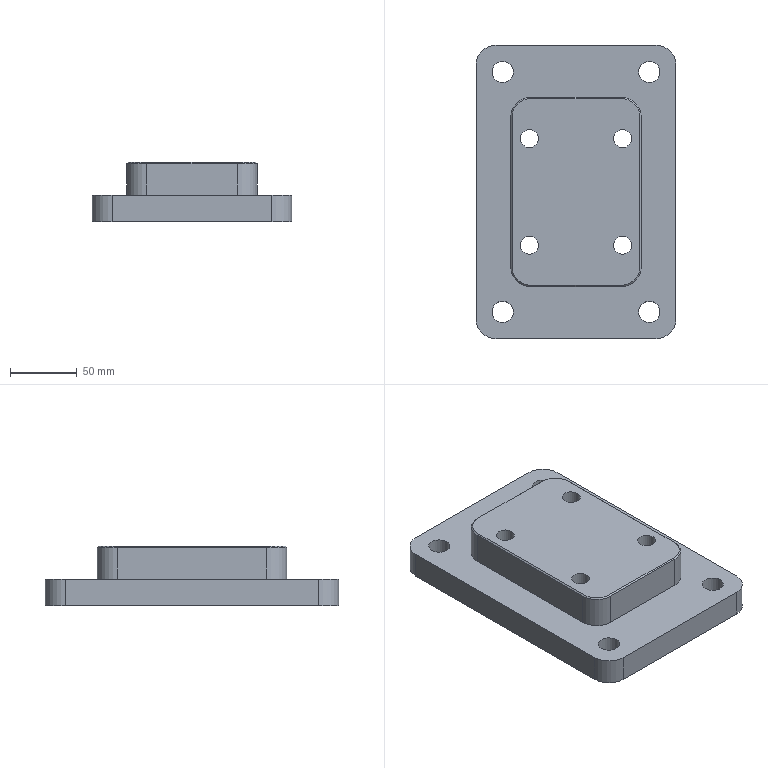NC program | NX | posted with a generic post | part box 150 x 220 x 45 mm
Lines 5642 to 5916 of 5916:
(HOLE_MILLING_COPY , TOOL : D10JING)
N11264 T11 M6
N11266 G54
N11268 G17 G0 G90 X-90. Y55. S5000 M3
N11270 G43 Z30. H11
N11272 Z0.5
N11274 G94 G3 X-88.5 Y56.5 R1.5 F1200.
N11276 X-90. Y58. R1.5
N11278 X-90. Y58. Z-4.5 I0. J-3.
N11280 X-90. Y58. Z-9.5 I0. J-3.
N11282 X-90. Y58. Z-14.5 I0. J-3.
N11284 X-90. Y58. Z-19.5 I0. J-3.
N11286 X-91.763 Y57.427 Z-20. R3.
N11288 X-92.427 Y53.237 R3.
N11290 X-91.763 Y57.427 R-3.
N11292 X-92.095 Y55.332 R1.5
N11294 X-90. Y55. R1.5
N11296 G0 Z30.
N11298 X-40. Y35.
N11300 Z0.5
N11302 G1 X-38.565 Y36.32
N11304 G3 X-40. Y40. R2.12
N11306 X-40. Y40. Z-4.5 I0. J-5.
N11308 X-40. Y40. Z-9.5 I0. J-5.
N11310 X-40. Y40. Z-14.5 I0. J-5.
N11312 X-35.245 Y33.455 Z-18. R-5.
N11314 X-38.455 Y39.755 R5.
N11316 X-35.245 Y33.455 R-5.
N11318 X-38.301 Y35.957 R2.12
N11320 G1 X-40. Y35.
N11322 G0 Z30.
N11324 X40.
N11326 Z0.5
N11328 G1 X41.435 Y36.32
N11330 G3 X40. Y40. R2.12
N11332 X40. Y40. Z-4.5 I0. J-5.
N11334 X40. Y40. Z-9.5 I0. J-5.
N11336 X40. Y40. Z-14.5 I0. J-5.
N11338 X44.755 Y33.455 Z-18. R-5.
N11340 X41.545 Y39.755 R5.
N11342 X44.755 Y33.455 R-5.
N11344 X41.699 Y35.957 R2.12
N11346 G1 X40. Y35.
N11348 G0 Z30.
N11350 X90. Y55.
N11352 Z0.5
N11354 G3 X91.5 Y56.5 R1.5
N11356 X90. Y58. R1.5
N11358 X90. Y58. Z-4.5 I0. J-3.
N11360 X90. Y58. Z-9.5 I0. J-3.
N11362 X90. Y58. Z-14.5 I0. J-3.
N11364 X90. Y58. Z-19.5 I0. J-3.
N11366 X88.237 Y57.427 Z-20. R3.
N11368 X87.573 Y53.237 R3.
N11370 X88.237 Y57.427 R-3.
N11372 X87.905 Y55.332 R1.5
N11374 X90. Y55. R1.5
N11376 G0 Z30.
N11378 Y-55.
N11380 Z0.5
N11382 G3 X91.5 Y-53.5 R1.5
N11384 X90. Y-52. R1.5
N11386 X90. Y-52. Z-4.5 I0. J-3.
N11388 X90. Y-52. Z-9.5 I0. J-3.
N11390 X90. Y-52. Z-14.5 I0. J-3.
N11392 X90. Y-52. Z-19.5 I0. J-3.
N11394 X88.237 Y-52.573 Z-20. R3.
N11396 X87.573 Y-56.763 R3.
N11398 X88.237 Y-52.573 R-3.
N11400 X87.905 Y-54.668 R1.5
N11402 X90. Y-55. R1.5
N11404 G0 Z30.
N11406 X40. Y-35.
N11408 Z0.5
N11410 G1 X41.435 Y-33.68
N11412 G3 X40. Y-30. R2.12
N11414 X40. Y-30. Z-4.5 I0. J-5.
N11416 X40. Y-30. Z-9.5 I0. J-5.
N11418 X40. Y-30. Z-14.5 I0. J-5.
N11420 X44.755 Y-36.545 Z-18. R-5.
N11422 X41.545 Y-30.245 R5.
N11424 X44.755 Y-36.545 R-5.
N11426 X41.699 Y-34.043 R2.12
N11428 G1 X40. Y-35.
N11430 G0 Z30.
N11432 X-40.
N11434 Z0.5
N11436 G1 X-38.565 Y-33.68
N11438 G3 X-40. Y-30. R2.12
N11440 X-40. Y-30. Z-4.5 I0. J-5.
N11442 X-40. Y-30. Z-9.5 I0. J-5.
N11444 X-40. Y-30. Z-14.5 I0. J-5.
N11446 X-35.245 Y-36.545 Z-18. R-5.
N11448 X-38.455 Y-30.245 R5.
N11450 X-35.245 Y-36.545 R-5.
N11452 X-38.301 Y-34.043 R2.12
N11454 G1 X-40. Y-35.
N11456 G0 Z30.
N11458 X-90. Y-55.
N11460 Z0.5
N11462 G3 X-88.5 Y-53.5 R1.5
N11464 X-90. Y-52. R1.5
N11466 X-90. Y-52. Z-4.5 I0. J-3.
N11468 X-90. Y-52. Z-9.5 I0. J-3.
N11470 X-90. Y-52. Z-14.5 I0. J-3.
N11472 X-90. Y-52. Z-19.5 I0. J-3.
N11474 X-91.763 Y-52.573 Z-20. R3.
N11476 X-92.427 Y-56.763 R3.
N11478 X-91.763 Y-52.573 R-3.
N11480 X-92.095 Y-54.668 R1.5
N11482 X-90. Y-55. R1.5
N11484 G0 Z30.
(ZLEVEL_PROFILE_1 , TOOL : D10JING)
N11486 X-87.875 Y-82.
N11488 Z-18.
N11490 G1 Z-20. F1250.
N11492 X-88.742 Y-80.499
N11494 G3 X-89.608 Y-80. R1.
N11496 G1 X-94.498
N11498 X-95.
N11500 G2 X-115. Y-60.012 R20.
N11502 G1 Y-59.981
N11504 Y-59.498
N11506 X-114.999 Y-59.053
N11508 Y-54.608
N11510 G3 X-115.499 Y-53.742 R1.
N11512 G1 X-117. Y-52.875
N11514 Z-18.
N11516 G0 Z30.
N11518 Y52.875
N11520 Z-18.
N11522 G1 Z-20.
N11524 X-115.499 Y53.742
N11526 G3 X-114.999 Y54.608 R1.
N11528 G1 Y59.053
N11530 X-115. Y59.498
N11532 Y60.
N11534 G2 X-95. Y80. R20.
N11536 G1 X-94.498
N11538 X-94.053 Y79.999
N11540 X-89.608
N11542 G3 X-88.742 Y80.499 R1.
N11544 G1 X-87.875 Y82.
N11546 Z-18.
N11548 G0 Z30.
N11550 X87.875
N11552 Z-18.
N11554 G1 Z-20.
N11556 X88.742 Y80.499
N11558 G3 X89.608 Y79.999 R1.
N11560 G1 X94.053
N11562 X94.498 Y80.
N11564 X95.
N11566 G2 X115. Y60. R20.
N11568 G1 Y59.498
N11570 Y54.608
N11572 G3 X115.499 Y53.742 R1.
N11574 G1 X117. Y52.875
N11576 Z-18.
N11578 G0 Z30.
N11580 Y-52.875
N11582 Z-18.
N11584 G1 Z-20.
N11586 X115.499 Y-53.742
N11588 G3 X115. Y-54.608 R1.
N11590 G1 Y-59.498
N11592 Y-60.
N11594 G2 X95. Y-80. R20.
N11596 G1 X94.498
N11598 X89.608
N11600 G3 X88.742 Y-80.499 R1.
N11602 G1 X87.875 Y-82.
N11604 Z-18.
N11606 G0 Z30.
N11608 M5
(PLANAR_MILL_COPY_COPY , TOOL : D6A45)
N11610 T07 M6
N11612 G54
N11614 G17 G0 G90 X90.766 Y61.343 S7500 M3
N11616 G43 Z30. H7
N11618 Z1.5
N11620 G94 G1 Z-1.5 F1250.
N11622 G3 X90. Y61.7 R1.
N11624 X83.3 Y55. R6.7
N11626 X90. Y61.7 R-6.7
N11628 X89.234 Y61.343 R1.
N11630 G1 Z1.5
N11632 G0 Z30.
N11634 X40.766 Y43.593
N11636 Z1.5
N11638 G1 Z-1.5
N11640 G3 X40. Y43.95 R1.
N11642 X31.05 Y35. R8.95
N11644 X40. Y43.95 R-8.95
N11646 X39.234 Y43.593 R1.
N11648 G1 Z1.5
N11650 G0 Z30.
N11652 X-39.234
N11654 Z1.5
N11656 G1 Z-1.5
N11658 G3 X-40. Y43.95 R1.
N11660 X-48.95 Y35. R8.95
N11662 X-40. Y43.95 R-8.95
N11664 X-40.766 Y43.593 R1.
N11666 G1 Z1.5
N11668 G0 Z30.
N11670 X-89.234 Y61.343
N11672 Z1.5
N11674 G1 Z-1.5
N11676 G3 X-90. Y61.7 R1.
N11678 X-96.7 Y55. R6.7
N11680 X-90. Y61.7 R-6.7
N11682 X-90.766 Y61.343 R1.
N11684 G1 Z1.5
N11686 G0 Z30.
N11688 X-96.343 Y-54.234
N11690 Z1.5
N11692 G1 Z-1.5
N11694 G3 X-96.7 Y-55. R1.
N11696 X-90. Y-61.7 R6.7
N11698 X-96.7 Y-55. R-6.7
N11700 X-96.343 Y-55.766 R1.
N11702 G1 Z1.5
N11704 G0 Z30.
N11706 X-40.766 Y-43.593
N11708 Z1.5
N11710 G1 Z-1.5
N11712 G3 X-40. Y-43.95 R1.
N11714 X-31.05 Y-35. R8.95
N11716 X-40. Y-43.95 R-8.95
N11718 X-39.234 Y-43.593 R1.
N11720 G1 Z1.5
N11722 G0 Z30.
N11724 X0.766 Y-76.657
N11726 Z1.5
N11728 G1 Z-1.5
N11730 G3 X0. Y-76.3 R1.
N11732 G1 X-95.
N11734 G2 X-111.3 Y-60. R16.3
N11736 G1 Y60.
N11738 G2 X-95. Y76.3 R16.3
N11740 G1 X95.
N11742 G2 X111.3 Y60. R16.3
N11744 G1 Y-60.
N11746 G2 X95. Y-76.3 R16.3
N11748 G1 X0.
N11750 G3 X-0.766 Y-76.657 R1.
N11752 G1 Z1.5
N11754 G0 Z30.
N11756 X39.234 Y-43.593
N11758 Z1.5
N11760 G1 Z-1.5
N11762 G3 X40. Y-43.95 R1.
N11764 X48.95 Y-35. R8.95
N11766 X40. Y-43.95 R-8.95
N11768 X40.766 Y-43.593 R1.
N11770 G1 Z1.5
N11772 G0 Z30.
N11774 X89.234 Y-61.343
N11776 Z1.5
N11778 G1 Z-1.5
N11780 G3 X90. Y-61.7 R1.
N11782 X96.7 Y-55. R6.7
N11784 X90. Y-61.7 R-6.7
N11786 X90.766 Y-61.343 R1.
N11788 G1 Z1.5
N11790 G0 Z30.
N11792 M5
N11794 M2